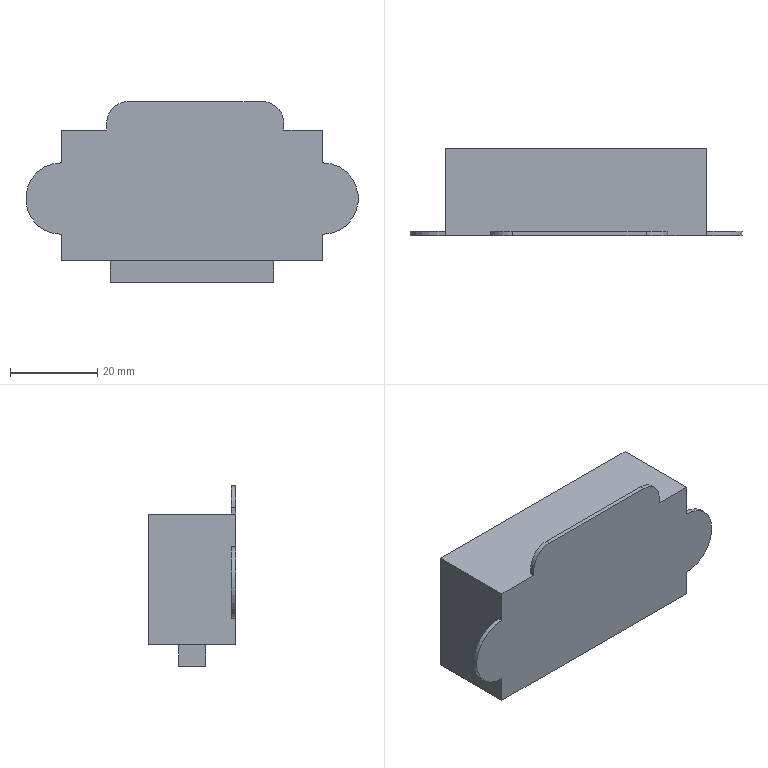Part | SolidWorks | features ICE 2, Extrusion 1 | 1 solid | 21 faces | box 76.413 x 20 x 41.556 mm | volume 37640 mm3 | plane 17 | cylinder 4 | commonest cylinder face diameters 10 x2 16.413 x2
STEP:
#1=CARTESIAN_POINT('',(-19.626,1.,15.));
#2=VERTEX_POINT('',#1);
#3=CARTESIAN_POINT('',(-19.626,0.,15.));
#4=VERTEX_POINT('',#3);
#5=CARTESIAN_POINT('',(-19.626,1.,15.));
#6=DIRECTION('',(0.,-1.,0.));
#7=VECTOR('',#6,1000.);
#8=LINE('',#5,#7);
#9=EDGE_CURVE('',#2,#4,#8,.T.);
#10=ORIENTED_EDGE('',*,*,#9,.F.);
#11=CARTESIAN_POINT('',(21.11,1.,15.));
#12=VERTEX_POINT('',#11);
#13=CARTESIAN_POINT('',(-19.626,1.,15.));
#14=DIRECTION('',(1.,0.,0.));
#15=VECTOR('',#14,1000.);
#16=LINE('',#13,#15);
#17=EDGE_CURVE('',#2,#12,#16,.T.);
#18=ORIENTED_EDGE('',*,*,#17,.T.);
#19=CARTESIAN_POINT('',(21.11,0.,15.));
#20=VERTEX_POINT('',#19);
#21=CARTESIAN_POINT('',(21.11,1.,15.));
#22=DIRECTION('',(0.,-1.,0.));
#23=VECTOR('',#22,1000.);
#24=LINE('',#21,#23);
#25=EDGE_CURVE('',#12,#20,#24,.T.);
#26=ORIENTED_EDGE('',*,*,#25,.T.);
#27=CARTESIAN_POINT('',(30.,0.,15.));
#28=VERTEX_POINT('',#27);
#29=CARTESIAN_POINT('',(-30.,0.,15.));
#30=DIRECTION('',(1.,0.,0.));
#31=VECTOR('',#30,1000.);
#32=LINE('',#29,#31);
#33=EDGE_CURVE('',#20,#28,#32,.T.);
#34=ORIENTED_EDGE('',*,*,#33,.T.);
#35=CARTESIAN_POINT('',(30.,20.,15.));
#36=VERTEX_POINT('',#35);
#37=CARTESIAN_POINT('',(30.,20.,15.));
#38=DIRECTION('',(0.,-1.,0.));
#39=VECTOR('',#38,1000.);
#40=LINE('',#37,#39);
#41=EDGE_CURVE('',#36,#28,#40,.T.);
#42=ORIENTED_EDGE('',*,*,#41,.F.);
#43=CARTESIAN_POINT('',(-30.,20.,15.));
#44=VERTEX_POINT('',#43);
#45=CARTESIAN_POINT('',(-30.,20.,15.));
#46=DIRECTION('',(1.,0.,0.));
#47=VECTOR('',#46,1000.);
#48=LINE('',#45,#47);
#49=EDGE_CURVE('',#44,#36,#48,.T.);
#50=ORIENTED_EDGE('',*,*,#49,.F.);
#51=CARTESIAN_POINT('',(-30.,0.,15.));
#52=VERTEX_POINT('',#51);
#53=CARTESIAN_POINT('',(-30.,20.,15.));
#54=DIRECTION('',(0.,-1.,0.));
#55=VECTOR('',#54,1000.);
#56=LINE('',#53,#55);
#57=EDGE_CURVE('',#44,#52,#56,.T.);
#58=ORIENTED_EDGE('',*,*,#57,.T.);
#59=CARTESIAN_POINT('',(-30.,0.,15.));
#60=DIRECTION('',(1.,0.,0.));
#61=VECTOR('',#60,1000.);
#62=LINE('',#59,#61);
#63=EDGE_CURVE('',#52,#4,#62,.T.);
#64=ORIENTED_EDGE('',*,*,#63,.T.);
#65=EDGE_LOOP('',(#10,#18,#26,#34,#42,#50,#58,#64));
#66=FACE_OUTER_BOUND('',#65,.T.);
#67=CARTESIAN_POINT('',(-30.,20.,15.));
#68=DIRECTION('',(0.,0.,-1.));
#69=DIRECTION('',(-1.,0.,0.));
#70=AXIS2_PLACEMENT_3D('',#67,#68,#69);
#71=PLANE('',#70);
#72=ADVANCED_FACE('',(#66),#71,.F.);
#73=CARTESIAN_POINT('',(30.,0.,-15.));
#74=VERTEX_POINT('',#73);
#75=CARTESIAN_POINT('',(-30.,0.,-15.));
#76=VERTEX_POINT('',#75);
#77=CARTESIAN_POINT('',(-30.,0.,-15.));
#78=DIRECTION('',(-1.,0.,0.));
#79=VECTOR('',#78,1000.);
#80=LINE('',#77,#79);
#81=EDGE_CURVE('',#74,#76,#80,.T.);
#82=ORIENTED_EDGE('',*,*,#81,.T.);
#83=CARTESIAN_POINT('',(-30.,20.,-15.));
#84=VERTEX_POINT('',#83);
#85=CARTESIAN_POINT('',(-30.,20.,-15.));
#86=DIRECTION('',(0.,-1.,0.));
#87=VECTOR('',#86,1000.);
#88=LINE('',#85,#87);
#89=EDGE_CURVE('',#84,#76,#88,.T.);
#90=ORIENTED_EDGE('',*,*,#89,.F.);
#91=CARTESIAN_POINT('',(30.,20.,-15.));
#92=VERTEX_POINT('',#91);
#93=CARTESIAN_POINT('',(-30.,20.,-15.));
#94=DIRECTION('',(-1.,0.,0.));
#95=VECTOR('',#94,1000.);
#96=LINE('',#93,#95);
#97=EDGE_CURVE('',#92,#84,#96,.T.);
#98=ORIENTED_EDGE('',*,*,#97,.F.);
#99=CARTESIAN_POINT('',(30.,20.,-15.));
#100=DIRECTION('',(0.,-1.,0.));
#101=VECTOR('',#100,1000.);
#102=LINE('',#99,#101);
#103=EDGE_CURVE('',#92,#74,#102,.T.);
#104=ORIENTED_EDGE('',*,*,#103,.T.);
#105=EDGE_LOOP('',(#82,#90,#98,#104));
#106=FACE_OUTER_BOUND('',#105,.T.);
#107=CARTESIAN_POINT('',(-18.753,6.813,-15.));
#108=VERTEX_POINT('',#107);
#109=CARTESIAN_POINT('',(-18.753,13.065,-15.));
#110=VERTEX_POINT('',#109);
#111=CARTESIAN_POINT('',(-18.753,6.813,-15.));
#112=DIRECTION('',(0.,1.,0.));
#113=VECTOR('',#112,1000.);
#114=LINE('',#111,#113);
#115=EDGE_CURVE('',#108,#110,#114,.T.);
#116=ORIENTED_EDGE('',*,*,#115,.F.);
#117=CARTESIAN_POINT('',(18.753,6.813,-15.));
#118=VERTEX_POINT('',#117);
#119=CARTESIAN_POINT('',(18.753,6.813,-15.));
#120=DIRECTION('',(-1.,0.,0.));
#121=VECTOR('',#120,1000.);
#122=LINE('',#119,#121);
#123=EDGE_CURVE('',#118,#108,#122,.T.);
#124=ORIENTED_EDGE('',*,*,#123,.F.);
#125=CARTESIAN_POINT('',(18.753,13.065,-15.));
#126=VERTEX_POINT('',#125);
#127=CARTESIAN_POINT('',(18.753,6.813,-15.));
#128=DIRECTION('',(0.,-1.,0.));
#129=VECTOR('',#128,1000.);
#130=LINE('',#127,#129);
#131=EDGE_CURVE('',#126,#118,#130,.T.);
#132=ORIENTED_EDGE('',*,*,#131,.F.);
#133=CARTESIAN_POINT('',(18.753,13.065,-15.));
#134=DIRECTION('',(1.,0.,0.));
#135=VECTOR('',#134,1000.);
#136=LINE('',#133,#135);
#137=EDGE_CURVE('',#110,#126,#136,.T.);
#138=ORIENTED_EDGE('',*,*,#137,.F.);
#139=EDGE_LOOP('',(#116,#124,#132,#138));
#140=FACE_BOUND('',#139,.T.);
#141=CARTESIAN_POINT('',(-30.,20.,-15.));
#142=DIRECTION('',(0.,0.,1.));
#143=DIRECTION('',(1.,0.,0.));
#144=AXIS2_PLACEMENT_3D('',#141,#142,#143);
#145=PLANE('',#144);
#146=ADVANCED_FACE('',(#106,#140),#145,.F.);
#147=CARTESIAN_POINT('',(30.,1.,7.473));
#148=VERTEX_POINT('',#147);
#149=CARTESIAN_POINT('',(30.,1.,-8.94));
#150=VERTEX_POINT('',#149);
#151=CARTESIAN_POINT('',(30.,1.,7.473));
#152=DIRECTION('',(0.,0.,-1.));
#153=VECTOR('',#152,1000.);
#154=LINE('',#151,#153);
#155=EDGE_CURVE('',#148,#150,#154,.T.);
#156=ORIENTED_EDGE('',*,*,#155,.T.);
#157=CARTESIAN_POINT('',(30.,0.,-8.94));
#158=VERTEX_POINT('',#157);
#159=CARTESIAN_POINT('',(30.,1.,-8.94));
#160=DIRECTION('',(0.,-1.,0.));
#161=VECTOR('',#160,1000.);
#162=LINE('',#159,#161);
#163=EDGE_CURVE('',#150,#158,#162,.T.);
#164=ORIENTED_EDGE('',*,*,#163,.T.);
#165=CARTESIAN_POINT('',(30.,0.,-15.));
#166=DIRECTION('',(0.,0.,-1.));
#167=VECTOR('',#166,1000.);
#168=LINE('',#165,#167);
#169=EDGE_CURVE('',#158,#74,#168,.T.);
#170=ORIENTED_EDGE('',*,*,#169,.T.);
#171=ORIENTED_EDGE('',*,*,#103,.F.);
#172=CARTESIAN_POINT('',(30.,20.,-15.));
#173=DIRECTION('',(0.,0.,-1.));
#174=VECTOR('',#173,1000.);
#175=LINE('',#172,#174);
#176=EDGE_CURVE('',#36,#92,#175,.T.);
#177=ORIENTED_EDGE('',*,*,#176,.F.);
#178=ORIENTED_EDGE('',*,*,#41,.T.);
#179=CARTESIAN_POINT('',(30.,0.,7.473));
#180=VERTEX_POINT('',#179);
#181=CARTESIAN_POINT('',(30.,0.,-15.));
#182=DIRECTION('',(0.,0.,-1.));
#183=VECTOR('',#182,1000.);
#184=LINE('',#181,#183);
#185=EDGE_CURVE('',#28,#180,#184,.T.);
#186=ORIENTED_EDGE('',*,*,#185,.T.);
#187=CARTESIAN_POINT('',(30.,1.,7.473));
#188=DIRECTION('',(0.,-1.,0.));
#189=VECTOR('',#188,1000.);
#190=LINE('',#187,#189);
#191=EDGE_CURVE('',#148,#180,#190,.T.);
#192=ORIENTED_EDGE('',*,*,#191,.F.);
#193=EDGE_LOOP('',(#156,#164,#170,#171,#177,#178,#186,#192));
#194=FACE_OUTER_BOUND('',#193,.T.);
#195=CARTESIAN_POINT('',(30.,20.,-15.));
#196=DIRECTION('',(-1.,0.,0.));
#197=DIRECTION('',(0.,0.,1.));
#198=AXIS2_PLACEMENT_3D('',#195,#196,#197);
#199=PLANE('',#198);
#200=ADVANCED_FACE('',(#194),#199,.F.);
#201=CARTESIAN_POINT('',(-30.,1.,-8.94));
#202=VERTEX_POINT('',#201);
#203=CARTESIAN_POINT('',(-30.,1.,7.473));
#204=VERTEX_POINT('',#203);
#205=CARTESIAN_POINT('',(-30.,1.,7.473));
#206=DIRECTION('',(0.,0.,1.));
#207=VECTOR('',#206,1000.);
#208=LINE('',#205,#207);
#209=EDGE_CURVE('',#202,#204,#208,.T.);
#210=ORIENTED_EDGE('',*,*,#209,.T.);
#211=CARTESIAN_POINT('',(-30.,0.,7.473));
#212=VERTEX_POINT('',#211);
#213=CARTESIAN_POINT('',(-30.,1.,7.473));
#214=DIRECTION('',(0.,-1.,0.));
#215=VECTOR('',#214,1000.);
#216=LINE('',#213,#215);
#217=EDGE_CURVE('',#204,#212,#216,.T.);
#218=ORIENTED_EDGE('',*,*,#217,.T.);
#219=CARTESIAN_POINT('',(-30.,0.,-15.));
#220=DIRECTION('',(0.,0.,1.));
#221=VECTOR('',#220,1000.);
#222=LINE('',#219,#221);
#223=EDGE_CURVE('',#212,#52,#222,.T.);
#224=ORIENTED_EDGE('',*,*,#223,.T.);
#225=ORIENTED_EDGE('',*,*,#57,.F.);
#226=CARTESIAN_POINT('',(-30.,20.,-15.));
#227=DIRECTION('',(0.,0.,1.));
#228=VECTOR('',#227,1000.);
#229=LINE('',#226,#228);
#230=EDGE_CURVE('',#84,#44,#229,.T.);
#231=ORIENTED_EDGE('',*,*,#230,.F.);
#232=ORIENTED_EDGE('',*,*,#89,.T.);
#233=CARTESIAN_POINT('',(-30.,0.,-8.94));
#234=VERTEX_POINT('',#233);
#235=CARTESIAN_POINT('',(-30.,0.,-15.));
#236=DIRECTION('',(0.,0.,1.));
#237=VECTOR('',#236,1000.);
#238=LINE('',#235,#237);
#239=EDGE_CURVE('',#76,#234,#238,.T.);
#240=ORIENTED_EDGE('',*,*,#239,.T.);
#241=CARTESIAN_POINT('',(-30.,1.,-8.94));
#242=DIRECTION('',(0.,-1.,0.));
#243=VECTOR('',#242,1000.);
#244=LINE('',#241,#243);
#245=EDGE_CURVE('',#202,#234,#244,.T.);
#246=ORIENTED_EDGE('',*,*,#245,.F.);
#247=EDGE_LOOP('',(#210,#218,#224,#225,#231,#232,#240,#246));
#248=FACE_OUTER_BOUND('',#247,.T.);
#249=CARTESIAN_POINT('',(-30.,20.,-15.));
#250=DIRECTION('',(1.,0.,0.));
#251=DIRECTION('',(0.,0.,-1.));
#252=AXIS2_PLACEMENT_3D('',#249,#250,#251);
#253=PLANE('',#252);
#254=ADVANCED_FACE('',(#248),#253,.F.);
#255=ORIENTED_EDGE('',*,*,#176,.T.);
#256=ORIENTED_EDGE('',*,*,#97,.T.);
#257=ORIENTED_EDGE('',*,*,#230,.T.);
#258=ORIENTED_EDGE('',*,*,#49,.T.);
#259=EDGE_LOOP('',(#255,#256,#257,#258));
#260=FACE_OUTER_BOUND('',#259,.T.);
#261=CARTESIAN_POINT('',(0.,20.,0.));
#262=DIRECTION('',(0.,1.,0.));
#263=DIRECTION('',(0.,0.,1.));
#264=AXIS2_PLACEMENT_3D('',#261,#262,#263);
#265=PLANE('',#264);
#266=ADVANCED_FACE('',(#260),#265,.T.);
#267=ORIENTED_EDGE('',*,*,#185,.F.);
#268=ORIENTED_EDGE('',*,*,#33,.F.);
#269=CARTESIAN_POINT('',(21.11,0.,16.556));
#270=VERTEX_POINT('',#269);
#271=CARTESIAN_POINT('',(21.11,0.,15.));
#272=DIRECTION('',(0.,0.,1.));
#273=VECTOR('',#272,1000.);
#274=LINE('',#271,#273);
#275=EDGE_CURVE('',#20,#270,#274,.T.);
#276=ORIENTED_EDGE('',*,*,#275,.T.);
#277=CARTESIAN_POINT('',(16.11,0.,21.556));
#278=VERTEX_POINT('',#277);
#279=CARTESIAN_POINT('',(16.11,0.,16.556));
#280=DIRECTION('',(0.,-1.,0.));
#281=DIRECTION('',(0.,0.,-1.));
#282=AXIS2_PLACEMENT_3D('',#279,#280,#281);
#283=CIRCLE('',#282,5.);
#284=EDGE_CURVE('',#270,#278,#283,.T.);
#285=ORIENTED_EDGE('',*,*,#284,.T.);
#286=CARTESIAN_POINT('',(-14.626,0.,21.556));
#287=VERTEX_POINT('',#286);
#288=CARTESIAN_POINT('',(-14.626,0.,21.556));
#289=DIRECTION('',(-1.,0.,0.));
#290=VECTOR('',#289,1000.);
#291=LINE('',#288,#290);
#292=EDGE_CURVE('',#278,#287,#291,.T.);
#293=ORIENTED_EDGE('',*,*,#292,.T.);
#294=CARTESIAN_POINT('',(-19.626,0.,16.556));
#295=VERTEX_POINT('',#294);
#296=CARTESIAN_POINT('',(-14.626,0.,16.556));
#297=DIRECTION('',(0.,-1.,0.));
#298=DIRECTION('',(0.,0.,1.));
#299=AXIS2_PLACEMENT_3D('',#296,#297,#298);
#300=CIRCLE('',#299,5.);
#301=EDGE_CURVE('',#287,#295,#300,.T.);
#302=ORIENTED_EDGE('',*,*,#301,.T.);
#303=CARTESIAN_POINT('',(-19.626,0.,15.));
#304=DIRECTION('',(0.,0.,-1.));
#305=VECTOR('',#304,1000.);
#306=LINE('',#303,#305);
#307=EDGE_CURVE('',#295,#4,#306,.T.);
#308=ORIENTED_EDGE('',*,*,#307,.T.);
#309=ORIENTED_EDGE('',*,*,#63,.F.);
#310=ORIENTED_EDGE('',*,*,#223,.F.);
#311=CARTESIAN_POINT('',(-30.,0.,-0.7334));
#312=DIRECTION('',(0.,-1.,0.));
#313=DIRECTION('',(0.,0.,-1.));
#314=AXIS2_PLACEMENT_3D('',#311,#312,#313);
#315=CIRCLE('',#314,8.206);
#316=EDGE_CURVE('',#212,#234,#315,.T.);
#317=ORIENTED_EDGE('',*,*,#316,.T.);
#318=ORIENTED_EDGE('',*,*,#239,.F.);
#319=ORIENTED_EDGE('',*,*,#81,.F.);
#320=ORIENTED_EDGE('',*,*,#169,.F.);
#321=CARTESIAN_POINT('',(30.,0.,-0.7334));
#322=DIRECTION('',(0.,-1.,0.));
#323=DIRECTION('',(0.,0.,1.));
#324=AXIS2_PLACEMENT_3D('',#321,#322,#323);
#325=CIRCLE('',#324,8.206);
#326=EDGE_CURVE('',#158,#180,#325,.T.);
#327=ORIENTED_EDGE('',*,*,#326,.T.);
#328=EDGE_LOOP('',(#267,#268,#276,#285,#293,#302,#308,#309,#310,#317,#318,#319,#320,#327));
#329=FACE_OUTER_BOUND('',#328,.T.);
#330=CARTESIAN_POINT('',(0.,0.,0.));
#331=DIRECTION('',(0.,1.,0.));
#332=DIRECTION('',(0.,0.,1.));
#333=AXIS2_PLACEMENT_3D('',#330,#331,#332);
#334=PLANE('',#333);
#335=ADVANCED_FACE('',(#329),#334,.F.);
#336=ORIENTED_EDGE('',*,*,#115,.T.);
#337=CARTESIAN_POINT('',(-18.753,13.065,-20.));
#338=VERTEX_POINT('',#337);
#339=CARTESIAN_POINT('',(-18.753,13.065,-20.));
#340=DIRECTION('',(0.,0.,1.));
#341=VECTOR('',#340,1000.);
#342=LINE('',#339,#341);
#343=EDGE_CURVE('',#338,#110,#342,.T.);
#344=ORIENTED_EDGE('',*,*,#343,.F.);
#345=CARTESIAN_POINT('',(-18.753,6.813,-20.));
#346=VERTEX_POINT('',#345);
#347=CARTESIAN_POINT('',(-18.753,6.813,-20.));
#348=DIRECTION('',(0.,1.,0.));
#349=VECTOR('',#348,1000.);
#350=LINE('',#347,#349);
#351=EDGE_CURVE('',#346,#338,#350,.T.);
#352=ORIENTED_EDGE('',*,*,#351,.F.);
#353=CARTESIAN_POINT('',(-18.753,6.813,-20.));
#354=DIRECTION('',(0.,0.,1.));
#355=VECTOR('',#354,1000.);
#356=LINE('',#353,#355);
#357=EDGE_CURVE('',#346,#108,#356,.T.);
#358=ORIENTED_EDGE('',*,*,#357,.T.);
#359=EDGE_LOOP('',(#336,#344,#352,#358));
#360=FACE_OUTER_BOUND('',#359,.T.);
#361=CARTESIAN_POINT('',(-18.753,6.813,-20.));
#362=DIRECTION('',(1.,0.,0.));
#363=DIRECTION('',(0.,0.,-1.));
#364=AXIS2_PLACEMENT_3D('',#361,#362,#363);
#365=PLANE('',#364);
#366=ADVANCED_FACE('',(#360),#365,.F.);
#367=ORIENTED_EDGE('',*,*,#137,.T.);
#368=CARTESIAN_POINT('',(18.753,13.065,-20.));
#369=VERTEX_POINT('',#368);
#370=CARTESIAN_POINT('',(18.753,13.065,-20.));
#371=DIRECTION('',(0.,0.,1.));
#372=VECTOR('',#371,1000.);
#373=LINE('',#370,#372);
#374=EDGE_CURVE('',#369,#126,#373,.T.);
#375=ORIENTED_EDGE('',*,*,#374,.F.);
#376=CARTESIAN_POINT('',(18.753,13.065,-20.));
#377=DIRECTION('',(1.,0.,0.));
#378=VECTOR('',#377,1000.);
#379=LINE('',#376,#378);
#380=EDGE_CURVE('',#338,#369,#379,.T.);
#381=ORIENTED_EDGE('',*,*,#380,.F.);
#382=ORIENTED_EDGE('',*,*,#343,.T.);
#383=EDGE_LOOP('',(#367,#375,#381,#382));
#384=FACE_OUTER_BOUND('',#383,.T.);
#385=CARTESIAN_POINT('',(18.753,13.065,-20.));
#386=DIRECTION('',(0.,-1.,0.));
#387=DIRECTION('',(0.,0.,-1.));
#388=AXIS2_PLACEMENT_3D('',#385,#386,#387);
#389=PLANE('',#388);
#390=ADVANCED_FACE('',(#384),#389,.F.);
#391=ORIENTED_EDGE('',*,*,#131,.T.);
#392=CARTESIAN_POINT('',(18.753,6.813,-20.));
#393=VERTEX_POINT('',#392);
#394=CARTESIAN_POINT('',(18.753,6.813,-20.));
#395=DIRECTION('',(0.,0.,1.));
#396=VECTOR('',#395,1000.);
#397=LINE('',#394,#396);
#398=EDGE_CURVE('',#393,#118,#397,.T.);
#399=ORIENTED_EDGE('',*,*,#398,.F.);
#400=CARTESIAN_POINT('',(18.753,6.813,-20.));
#401=DIRECTION('',(0.,-1.,0.));
#402=VECTOR('',#401,1000.);
#403=LINE('',#400,#402);
#404=EDGE_CURVE('',#369,#393,#403,.T.);
#405=ORIENTED_EDGE('',*,*,#404,.F.);
#406=ORIENTED_EDGE('',*,*,#374,.T.);
#407=EDGE_LOOP('',(#391,#399,#405,#406));
#408=FACE_OUTER_BOUND('',#407,.T.);
#409=CARTESIAN_POINT('',(18.753,6.813,-20.));
#410=DIRECTION('',(-1.,0.,0.));
#411=DIRECTION('',(0.,-1.,0.));
#412=AXIS2_PLACEMENT_3D('',#409,#410,#411);
#413=PLANE('',#412);
#414=ADVANCED_FACE('',(#408),#413,.F.);
#415=ORIENTED_EDGE('',*,*,#123,.T.);
#416=ORIENTED_EDGE('',*,*,#357,.F.);
#417=CARTESIAN_POINT('',(18.753,6.813,-20.));
#418=DIRECTION('',(-1.,0.,0.));
#419=VECTOR('',#418,1000.);
#420=LINE('',#417,#419);
#421=EDGE_CURVE('',#393,#346,#420,.T.);
#422=ORIENTED_EDGE('',*,*,#421,.F.);
#423=ORIENTED_EDGE('',*,*,#398,.T.);
#424=EDGE_LOOP('',(#415,#416,#422,#423));
#425=FACE_OUTER_BOUND('',#424,.T.);
#426=CARTESIAN_POINT('',(18.753,6.813,-20.));
#427=DIRECTION('',(0.,1.,0.));
#428=DIRECTION('',(0.,0.,1.));
#429=AXIS2_PLACEMENT_3D('',#426,#427,#428);
#430=PLANE('',#429);
#431=ADVANCED_FACE('',(#425),#430,.F.);
#432=ORIENTED_EDGE('',*,*,#351,.T.);
#433=ORIENTED_EDGE('',*,*,#380,.T.);
#434=ORIENTED_EDGE('',*,*,#404,.T.);
#435=ORIENTED_EDGE('',*,*,#421,.T.);
#436=EDGE_LOOP('',(#432,#433,#434,#435));
#437=FACE_OUTER_BOUND('',#436,.T.);
#438=CARTESIAN_POINT('',(0.,0.,-20.));
#439=DIRECTION('',(0.,0.,1.));
#440=DIRECTION('',(1.,0.,0.));
#441=AXIS2_PLACEMENT_3D('',#438,#439,#440);
#442=PLANE('',#441);
#443=ADVANCED_FACE('',(#437),#442,.F.);
#444=ORIENTED_EDGE('',*,*,#316,.F.);
#445=ORIENTED_EDGE('',*,*,#217,.F.);
#446=CARTESIAN_POINT('',(-30.,1.,-0.7334));
#447=DIRECTION('',(0.,-1.,0.));
#448=DIRECTION('',(0.,0.,-1.));
#449=AXIS2_PLACEMENT_3D('',#446,#447,#448);
#450=CIRCLE('',#449,8.206);
#451=EDGE_CURVE('',#204,#202,#450,.T.);
#452=ORIENTED_EDGE('',*,*,#451,.T.);
#453=ORIENTED_EDGE('',*,*,#245,.T.);
#454=EDGE_LOOP('',(#444,#445,#452,#453));
#455=FACE_OUTER_BOUND('',#454,.T.);
#456=CARTESIAN_POINT('',(-30.,1.,-0.7334));
#457=DIRECTION('',(0.,-1.,0.));
#458=DIRECTION('',(0.,0.,-1.));
#459=AXIS2_PLACEMENT_3D('',#456,#457,#458);
#460=CYLINDRICAL_SURFACE('',#459,8.206);
#461=ADVANCED_FACE('',(#455),#460,.T.);
#462=ORIENTED_EDGE('',*,*,#451,.F.);
#463=ORIENTED_EDGE('',*,*,#209,.F.);
#464=EDGE_LOOP('',(#462,#463));
#465=FACE_OUTER_BOUND('',#464,.T.);
#466=CARTESIAN_POINT('',(-30.,1.,-0.7334));
#467=DIRECTION('',(0.,-1.,0.));
#468=DIRECTION('',(0.,0.,-1.));
#469=AXIS2_PLACEMENT_3D('',#466,#467,#468);
#470=PLANE('',#469);
#471=ADVANCED_FACE('',(#465),#470,.F.);
#472=ORIENTED_EDGE('',*,*,#326,.F.);
#473=ORIENTED_EDGE('',*,*,#163,.F.);
#474=CARTESIAN_POINT('',(30.,1.,-0.7334));
#475=DIRECTION('',(0.,-1.,0.));
#476=DIRECTION('',(0.,0.,1.));
#477=AXIS2_PLACEMENT_3D('',#474,#475,#476);
#478=CIRCLE('',#477,8.206);
#479=EDGE_CURVE('',#150,#148,#478,.T.);
#480=ORIENTED_EDGE('',*,*,#479,.T.);
#481=ORIENTED_EDGE('',*,*,#191,.T.);
#482=EDGE_LOOP('',(#472,#473,#480,#481));
#483=FACE_OUTER_BOUND('',#482,.T.);
#484=CARTESIAN_POINT('',(30.,1.,-0.7334));
#485=DIRECTION('',(0.,-1.,0.));
#486=DIRECTION('',(0.,0.,-1.));
#487=AXIS2_PLACEMENT_3D('',#484,#485,#486);
#488=CYLINDRICAL_SURFACE('',#487,8.206);
#489=ADVANCED_FACE('',(#483),#488,.T.);
#490=ORIENTED_EDGE('',*,*,#479,.F.);
#491=ORIENTED_EDGE('',*,*,#155,.F.);
#492=EDGE_LOOP('',(#490,#491));
#493=FACE_OUTER_BOUND('',#492,.T.);
#494=CARTESIAN_POINT('',(30.,1.,-0.7334));
#495=DIRECTION('',(0.,1.,0.));
#496=DIRECTION('',(0.,0.,1.));
#497=AXIS2_PLACEMENT_3D('',#494,#495,#496);
#498=PLANE('',#497);
#499=ADVANCED_FACE('',(#493),#498,.T.);
#500=ORIENTED_EDGE('',*,*,#307,.F.);
#501=CARTESIAN_POINT('',(-19.626,1.,16.556));
#502=VERTEX_POINT('',#501);
#503=CARTESIAN_POINT('',(-19.626,1.,16.556));
#504=DIRECTION('',(0.,-1.,0.));
#505=VECTOR('',#504,1000.);
#506=LINE('',#503,#505);
#507=EDGE_CURVE('',#502,#295,#506,.T.);
#508=ORIENTED_EDGE('',*,*,#507,.F.);
#509=CARTESIAN_POINT('',(-19.626,1.,15.));
#510=DIRECTION('',(0.,0.,-1.));
#511=VECTOR('',#510,1000.);
#512=LINE('',#509,#511);
#513=EDGE_CURVE('',#502,#2,#512,.T.);
#514=ORIENTED_EDGE('',*,*,#513,.T.);
#515=ORIENTED_EDGE('',*,*,#9,.T.);
#516=EDGE_LOOP('',(#500,#508,#514,#515));
#517=FACE_OUTER_BOUND('',#516,.T.);
#518=CARTESIAN_POINT('',(-19.626,1.,15.));
#519=DIRECTION('',(-1.,0.,0.));
#520=DIRECTION('',(0.,0.,1.));
#521=AXIS2_PLACEMENT_3D('',#518,#519,#520);
#522=PLANE('',#521);
#523=ADVANCED_FACE('',(#517),#522,.T.);
#524=ORIENTED_EDGE('',*,*,#301,.F.);
#525=CARTESIAN_POINT('',(-14.626,1.,21.556));
#526=VERTEX_POINT('',#525);
#527=CARTESIAN_POINT('',(-14.626,1.,21.556));
#528=DIRECTION('',(0.,-1.,0.));
#529=VECTOR('',#528,1000.);
#530=LINE('',#527,#529);
#531=EDGE_CURVE('',#526,#287,#530,.T.);
#532=ORIENTED_EDGE('',*,*,#531,.F.);
#533=CARTESIAN_POINT('',(-14.626,1.,16.556));
#534=DIRECTION('',(0.,-1.,0.));
#535=DIRECTION('',(0.,0.,1.));
#536=AXIS2_PLACEMENT_3D('',#533,#534,#535);
#537=CIRCLE('',#536,5.);
#538=EDGE_CURVE('',#526,#502,#537,.T.);
#539=ORIENTED_EDGE('',*,*,#538,.T.);
#540=ORIENTED_EDGE('',*,*,#507,.T.);
#541=EDGE_LOOP('',(#524,#532,#539,#540));
#542=FACE_OUTER_BOUND('',#541,.T.);
#543=CARTESIAN_POINT('',(-14.626,1.,16.556));
#544=DIRECTION('',(0.,-1.,0.));
#545=DIRECTION('',(0.,0.,-1.));
#546=AXIS2_PLACEMENT_3D('',#543,#544,#545);
#547=CYLINDRICAL_SURFACE('',#546,5.);
#548=ADVANCED_FACE('',(#542),#547,.T.);
#549=ORIENTED_EDGE('',*,*,#292,.F.);
#550=CARTESIAN_POINT('',(16.11,1.,21.556));
#551=VERTEX_POINT('',#550);
#552=CARTESIAN_POINT('',(16.11,1.,21.556));
#553=DIRECTION('',(0.,-1.,0.));
#554=VECTOR('',#553,1000.);
#555=LINE('',#552,#554);
#556=EDGE_CURVE('',#551,#278,#555,.T.);
#557=ORIENTED_EDGE('',*,*,#556,.F.);
#558=CARTESIAN_POINT('',(-14.626,1.,21.556));
#559=DIRECTION('',(-1.,0.,0.));
#560=VECTOR('',#559,1000.);
#561=LINE('',#558,#560);
#562=EDGE_CURVE('',#551,#526,#561,.T.);
#563=ORIENTED_EDGE('',*,*,#562,.T.);
#564=ORIENTED_EDGE('',*,*,#531,.T.);
#565=EDGE_LOOP('',(#549,#557,#563,#564));
#566=FACE_OUTER_BOUND('',#565,.T.);
#567=CARTESIAN_POINT('',(-14.626,1.,21.556));
#568=DIRECTION('',(0.,0.,1.));
#569=DIRECTION('',(1.,0.,0.));
#570=AXIS2_PLACEMENT_3D('',#567,#568,#569);
#571=PLANE('',#570);
#572=ADVANCED_FACE('',(#566),#571,.T.);
#573=ORIENTED_EDGE('',*,*,#284,.F.);
#574=CARTESIAN_POINT('',(21.11,1.,16.556));
#575=VERTEX_POINT('',#574);
#576=CARTESIAN_POINT('',(21.11,1.,16.556));
#577=DIRECTION('',(0.,-1.,0.));
#578=VECTOR('',#577,1000.);
#579=LINE('',#576,#578);
#580=EDGE_CURVE('',#575,#270,#579,.T.);
#581=ORIENTED_EDGE('',*,*,#580,.F.);
#582=CARTESIAN_POINT('',(16.11,1.,16.556));
#583=DIRECTION('',(0.,-1.,0.));
#584=DIRECTION('',(0.,0.,-1.));
#585=AXIS2_PLACEMENT_3D('',#582,#583,#584);
#586=CIRCLE('',#585,5.);
#587=EDGE_CURVE('',#575,#551,#586,.T.);
#588=ORIENTED_EDGE('',*,*,#587,.T.);
#589=ORIENTED_EDGE('',*,*,#556,.T.);
#590=EDGE_LOOP('',(#573,#581,#588,#589));
#591=FACE_OUTER_BOUND('',#590,.T.);
#592=CARTESIAN_POINT('',(16.11,1.,16.556));
#593=DIRECTION('',(0.,-1.,0.));
#594=DIRECTION('',(0.,0.,-1.));
#595=AXIS2_PLACEMENT_3D('',#592,#593,#594);
#596=CYLINDRICAL_SURFACE('',#595,5.);
#597=ADVANCED_FACE('',(#591),#596,.T.);
#598=ORIENTED_EDGE('',*,*,#275,.F.);
#599=ORIENTED_EDGE('',*,*,#25,.F.);
#600=CARTESIAN_POINT('',(21.11,1.,15.));
#601=DIRECTION('',(0.,0.,1.));
#602=VECTOR('',#601,1000.);
#603=LINE('',#600,#602);
#604=EDGE_CURVE('',#12,#575,#603,.T.);
#605=ORIENTED_EDGE('',*,*,#604,.T.);
#606=ORIENTED_EDGE('',*,*,#580,.T.);
#607=EDGE_LOOP('',(#598,#599,#605,#606));
#608=FACE_OUTER_BOUND('',#607,.T.);
#609=CARTESIAN_POINT('',(21.11,1.,15.));
#610=DIRECTION('',(1.,0.,0.));
#611=DIRECTION('',(0.,0.,-1.));
#612=AXIS2_PLACEMENT_3D('',#609,#610,#611);
#613=PLANE('',#612);
#614=ADVANCED_FACE('',(#608),#613,.T.);
#615=ORIENTED_EDGE('',*,*,#513,.F.);
#616=ORIENTED_EDGE('',*,*,#538,.F.);
#617=ORIENTED_EDGE('',*,*,#562,.F.);
#618=ORIENTED_EDGE('',*,*,#587,.F.);
#619=ORIENTED_EDGE('',*,*,#604,.F.);
#620=ORIENTED_EDGE('',*,*,#17,.F.);
#621=EDGE_LOOP('',(#615,#616,#617,#618,#619,#620));
#622=FACE_OUTER_BOUND('',#621,.T.);
#623=CARTESIAN_POINT('',(-14.626,1.,16.556));
#624=DIRECTION('',(0.,1.,0.));
#625=DIRECTION('',(0.,0.,1.));
#626=AXIS2_PLACEMENT_3D('',#623,#624,#625);
#627=PLANE('',#626);
#628=ADVANCED_FACE('',(#622),#627,.T.);
#629=CLOSED_SHELL('',(#72,#146,#200,#254,#266,#335,#366,#390,#414,#431,#443,#461,#471,#489,#499,#523,#548,#572,#597,#614,#628));
#630=MANIFOLD_SOLID_BREP('',#629);
#631=CARTESIAN_POINT('',(0.,0.,0.));
#632=DIRECTION('',(0.,0.,1.));
#633=DIRECTION('',(1.,0.,0.));
#634=AXIS2_PLACEMENT_3D('',#631,#632,#633);
#635=(LENGTH_UNIT()NAMED_UNIT(*)SI_UNIT(.MILLI.,.METRE.));
#636=UNCERTAINTY_MEASURE_WITH_UNIT(LENGTH_MEASURE(0.00001),#635,'','');
#637=(NAMED_UNIT(*)PLANE_ANGLE_UNIT()SI_UNIT($,.RADIAN.));
#638=(NAMED_UNIT(*)SI_UNIT($,.STERADIAN.)SOLID_ANGLE_UNIT());
#639=(GEOMETRIC_REPRESENTATION_CONTEXT(3)GLOBAL_UNCERTAINTY_ASSIGNED_CONTEXT((#636))GLOBAL_UNIT_ASSIGNED_CONTEXT((#635,#637,#638))REPRESENTATION_CONTEXT('',''));
#640=ADVANCED_BREP_SHAPE_REPRESENTATION('',(#630,#634),#639);